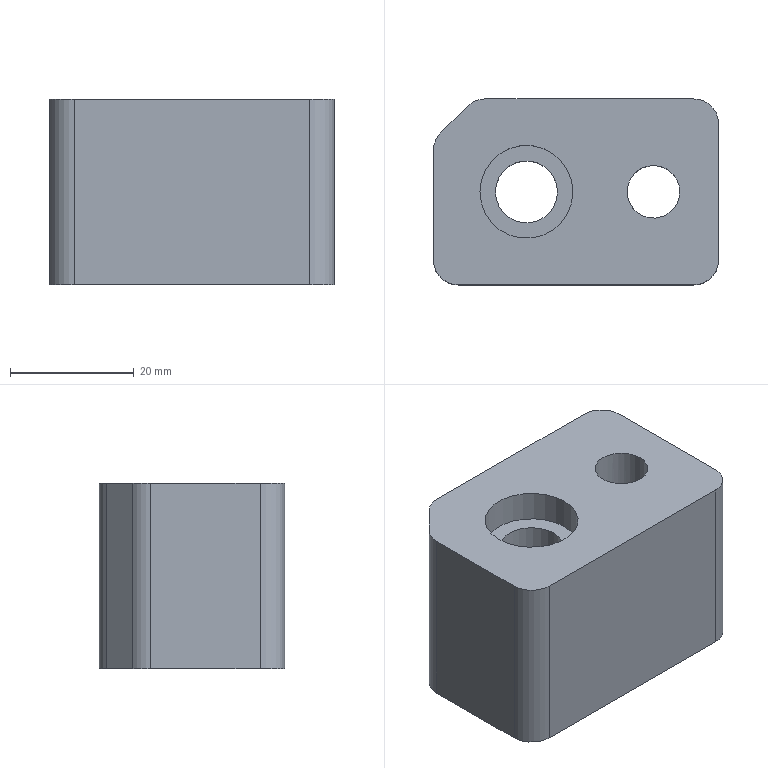Part | NX | features 7 2 | 1 solid | 18 faces | box 46 x 30 x 30 mm | volume 34235 mm3 | plane 9 | cylinder 9 | commonest cylinder face diameters 8 x5 8.5 x1 10 x1 14.5 x1 15 x1
STEP:
#1=CARTESIAN_POINT('',(3297.747,77.328,91.));
#2=VERTEX_POINT('',#1);
#3=CARTESIAN_POINT('',(3290.247,77.328,91.));
#4=DIRECTION('',(0.,0.,1.));
#5=DIRECTION('',(1.,0.,0.));
#6=AXIS2_PLACEMENT_3D('',#3,#4,#5);
#7=CIRCLE('',#6,7.5);
#8=EDGE_CURVE('',#2,#2,#7,.T.);
#9=ORIENTED_EDGE('',*,*,#8,.F.);
#10=EDGE_LOOP('',(#9));
#11=FACE_BOUND('',#10,.T.);
#12=CARTESIAN_POINT('',(3317.247,62.328,91.));
#13=VERTEX_POINT('',#12);
#14=CARTESIAN_POINT('',(3279.247,62.328,91.));
#15=VERTEX_POINT('',#14);
#16=CARTESIAN_POINT('',(3290.247,62.328,91.));
#17=DIRECTION('',(-1.,0.,0.));
#18=VECTOR('',#17,1000.);
#19=LINE('',#16,#18);
#20=EDGE_CURVE('',#13,#15,#19,.T.);
#21=ORIENTED_EDGE('',*,*,#20,.F.);
#22=CARTESIAN_POINT('',(3321.247,66.328,91.));
#23=VERTEX_POINT('',#22);
#24=CARTESIAN_POINT('',(3317.247,66.328,91.));
#25=DIRECTION('',(0.,0.,1.));
#26=DIRECTION('',(0.,1.,0.));
#27=AXIS2_PLACEMENT_3D('',#24,#25,#26);
#28=CIRCLE('',#27,4.);
#29=EDGE_CURVE('',#13,#23,#28,.T.);
#30=ORIENTED_EDGE('',*,*,#29,.T.);
#31=CARTESIAN_POINT('',(3321.247,88.328,91.));
#32=VERTEX_POINT('',#31);
#33=CARTESIAN_POINT('',(3321.247,77.328,91.));
#34=DIRECTION('',(0.,-1.,0.));
#35=VECTOR('',#34,1000.);
#36=LINE('',#33,#35);
#37=EDGE_CURVE('',#32,#23,#36,.T.);
#38=ORIENTED_EDGE('',*,*,#37,.F.);
#39=CARTESIAN_POINT('',(3317.247,92.328,91.));
#40=VERTEX_POINT('',#39);
#41=CARTESIAN_POINT('',(3317.247,88.328,91.));
#42=DIRECTION('',(0.,0.,1.));
#43=DIRECTION('',(0.,1.,0.));
#44=AXIS2_PLACEMENT_3D('',#41,#42,#43);
#45=CIRCLE('',#44,4.);
#46=EDGE_CURVE('',#32,#40,#45,.T.);
#47=ORIENTED_EDGE('',*,*,#46,.T.);
#48=CARTESIAN_POINT('',(3283.54,92.328,91.));
#49=VERTEX_POINT('',#48);
#50=CARTESIAN_POINT('',(3290.247,92.328,91.));
#51=DIRECTION('',(1.,0.,0.));
#52=VECTOR('',#51,1000.);
#53=LINE('',#50,#52);
#54=EDGE_CURVE('',#49,#40,#53,.T.);
#55=ORIENTED_EDGE('',*,*,#54,.F.);
#56=CARTESIAN_POINT('',(3280.711,91.157,91.));
#57=VERTEX_POINT('',#56);
#58=CARTESIAN_POINT('',(3283.54,88.328,91.));
#59=DIRECTION('',(0.,0.,1.));
#60=DIRECTION('',(0.,1.,0.));
#61=AXIS2_PLACEMENT_3D('',#58,#59,#60);
#62=CIRCLE('',#61,4.);
#63=EDGE_CURVE('',#49,#57,#62,.T.);
#64=ORIENTED_EDGE('',*,*,#63,.T.);
#65=CARTESIAN_POINT('',(3276.419,86.864,91.));
#66=VERTEX_POINT('',#65);
#67=CARTESIAN_POINT('',(3279.815,90.26,91.));
#68=DIRECTION('',(-0.7071,-0.7071,0.));
#69=VECTOR('',#68,1000.);
#70=LINE('',#67,#69);
#71=EDGE_CURVE('',#57,#66,#70,.T.);
#72=ORIENTED_EDGE('',*,*,#71,.T.);
#73=CARTESIAN_POINT('',(3275.247,84.035,91.));
#74=VERTEX_POINT('',#73);
#75=CARTESIAN_POINT('',(3279.247,84.035,91.));
#76=DIRECTION('',(0.,0.,1.));
#77=DIRECTION('',(0.,1.,0.));
#78=AXIS2_PLACEMENT_3D('',#75,#76,#77);
#79=CIRCLE('',#78,4.);
#80=EDGE_CURVE('',#66,#74,#79,.T.);
#81=ORIENTED_EDGE('',*,*,#80,.T.);
#82=CARTESIAN_POINT('',(3275.247,66.328,91.));
#83=VERTEX_POINT('',#82);
#84=CARTESIAN_POINT('',(3275.247,77.328,91.));
#85=DIRECTION('',(0.,1.,0.));
#86=VECTOR('',#85,1000.);
#87=LINE('',#84,#86);
#88=EDGE_CURVE('',#83,#74,#87,.T.);
#89=ORIENTED_EDGE('',*,*,#88,.F.);
#90=CARTESIAN_POINT('',(3279.247,66.328,91.));
#91=DIRECTION('',(0.,0.,1.));
#92=DIRECTION('',(0.,1.,0.));
#93=AXIS2_PLACEMENT_3D('',#90,#91,#92);
#94=CIRCLE('',#93,4.);
#95=EDGE_CURVE('',#83,#15,#94,.T.);
#96=ORIENTED_EDGE('',*,*,#95,.T.);
#97=EDGE_LOOP('',(#21,#30,#38,#47,#55,#64,#72,#81,#89,#96));
#98=FACE_BOUND('',#97,.T.);
#99=CARTESIAN_POINT('',(3310.747,81.578,91.));
#100=VERTEX_POINT('',#99);
#101=CARTESIAN_POINT('',(3310.747,77.328,91.));
#102=DIRECTION('',(0.,0.,-1.));
#103=DIRECTION('',(0.,1.,0.));
#104=AXIS2_PLACEMENT_3D('',#101,#102,#103);
#105=CIRCLE('',#104,4.25);
#106=EDGE_CURVE('',#100,#100,#105,.T.);
#107=ORIENTED_EDGE('',*,*,#106,.T.);
#108=EDGE_LOOP('',(#107));
#109=FACE_BOUND('',#108,.T.);
#110=CARTESIAN_POINT('',(3292.747,77.328,91.));
#111=DIRECTION('',(0.,0.,1.));
#112=DIRECTION('',(0.,-1.,0.));
#113=AXIS2_PLACEMENT_3D('',#110,#111,#112);
#114=PLANE('',#113);
#115=ADVANCED_FACE('',(#11,#98,#109),#114,.T.);
#116=CARTESIAN_POINT('',(3285.247,77.328,61.));
#117=VERTEX_POINT('',#116);
#118=CARTESIAN_POINT('',(3290.247,77.328,61.));
#119=DIRECTION('',(0.,0.,-1.));
#120=DIRECTION('',(-1.,0.,0.));
#121=AXIS2_PLACEMENT_3D('',#118,#119,#120);
#122=CIRCLE('',#121,5.);
#123=EDGE_CURVE('',#117,#117,#122,.T.);
#124=ORIENTED_EDGE('',*,*,#123,.F.);
#125=EDGE_LOOP('',(#124));
#126=FACE_BOUND('',#125,.T.);
#127=CARTESIAN_POINT('',(3303.497,77.328,61.));
#128=VERTEX_POINT('',#127);
#129=CARTESIAN_POINT('',(3310.747,77.328,61.));
#130=DIRECTION('',(0.,0.,-1.));
#131=DIRECTION('',(-1.,0.,0.));
#132=AXIS2_PLACEMENT_3D('',#129,#130,#131);
#133=CIRCLE('',#132,7.25);
#134=EDGE_CURVE('',#128,#128,#133,.T.);
#135=ORIENTED_EDGE('',*,*,#134,.F.);
#136=EDGE_LOOP('',(#135));
#137=FACE_BOUND('',#136,.T.);
#138=CARTESIAN_POINT('',(3321.247,66.328,61.));
#139=VERTEX_POINT('',#138);
#140=CARTESIAN_POINT('',(3321.247,88.328,61.));
#141=VERTEX_POINT('',#140);
#142=CARTESIAN_POINT('',(3321.247,-99.672,61.));
#143=DIRECTION('',(0.,1.,0.));
#144=VECTOR('',#143,1000.);
#145=LINE('',#142,#144);
#146=EDGE_CURVE('',#139,#141,#145,.T.);
#147=ORIENTED_EDGE('',*,*,#146,.F.);
#148=CARTESIAN_POINT('',(3317.247,62.328,61.));
#149=VERTEX_POINT('',#148);
#150=CARTESIAN_POINT('',(3317.247,66.328,61.));
#151=DIRECTION('',(0.,0.,-1.));
#152=DIRECTION('',(-1.,0.,0.));
#153=AXIS2_PLACEMENT_3D('',#150,#151,#152);
#154=CIRCLE('',#153,4.);
#155=EDGE_CURVE('',#139,#149,#154,.T.);
#156=ORIENTED_EDGE('',*,*,#155,.T.);
#157=CARTESIAN_POINT('',(3279.247,62.328,61.));
#158=VERTEX_POINT('',#157);
#159=CARTESIAN_POINT('',(3475.247,62.328,61.));
#160=DIRECTION('',(1.,0.,0.));
#161=VECTOR('',#160,1000.);
#162=LINE('',#159,#161);
#163=EDGE_CURVE('',#158,#149,#162,.T.);
#164=ORIENTED_EDGE('',*,*,#163,.F.);
#165=CARTESIAN_POINT('',(3275.247,66.328,61.));
#166=VERTEX_POINT('',#165);
#167=CARTESIAN_POINT('',(3279.247,66.328,61.));
#168=DIRECTION('',(0.,0.,-1.));
#169=DIRECTION('',(-1.,0.,0.));
#170=AXIS2_PLACEMENT_3D('',#167,#168,#169);
#171=CIRCLE('',#170,4.);
#172=EDGE_CURVE('',#158,#166,#171,.T.);
#173=ORIENTED_EDGE('',*,*,#172,.T.);
#174=CARTESIAN_POINT('',(3275.247,84.035,61.));
#175=VERTEX_POINT('',#174);
#176=CARTESIAN_POINT('',(3275.247,-99.672,61.));
#177=DIRECTION('',(0.,-1.,0.));
#178=VECTOR('',#177,1000.);
#179=LINE('',#176,#178);
#180=EDGE_CURVE('',#175,#166,#179,.T.);
#181=ORIENTED_EDGE('',*,*,#180,.F.);
#182=CARTESIAN_POINT('',(3276.419,86.864,61.));
#183=VERTEX_POINT('',#182);
#184=CARTESIAN_POINT('',(3279.247,84.035,61.));
#185=DIRECTION('',(0.,0.,-1.));
#186=DIRECTION('',(-1.,0.,0.));
#187=AXIS2_PLACEMENT_3D('',#184,#185,#186);
#188=CIRCLE('',#187,4.);
#189=EDGE_CURVE('',#175,#183,#188,.T.);
#190=ORIENTED_EDGE('',*,*,#189,.T.);
#191=CARTESIAN_POINT('',(3280.711,91.157,61.));
#192=VERTEX_POINT('',#191);
#193=CARTESIAN_POINT('',(3282.565,93.01,61.));
#194=DIRECTION('',(0.7071,0.7071,0.));
#195=VECTOR('',#194,1000.);
#196=LINE('',#193,#195);
#197=EDGE_CURVE('',#183,#192,#196,.T.);
#198=ORIENTED_EDGE('',*,*,#197,.T.);
#199=CARTESIAN_POINT('',(3283.54,92.328,61.));
#200=VERTEX_POINT('',#199);
#201=CARTESIAN_POINT('',(3283.54,88.328,61.));
#202=DIRECTION('',(0.,0.,-1.));
#203=DIRECTION('',(-1.,0.,0.));
#204=AXIS2_PLACEMENT_3D('',#201,#202,#203);
#205=CIRCLE('',#204,4.);
#206=EDGE_CURVE('',#192,#200,#205,.T.);
#207=ORIENTED_EDGE('',*,*,#206,.T.);
#208=CARTESIAN_POINT('',(3317.247,92.328,61.));
#209=VERTEX_POINT('',#208);
#210=CARTESIAN_POINT('',(3475.247,92.328,61.));
#211=DIRECTION('',(-1.,0.,0.));
#212=VECTOR('',#211,1000.);
#213=LINE('',#210,#212);
#214=EDGE_CURVE('',#209,#200,#213,.T.);
#215=ORIENTED_EDGE('',*,*,#214,.F.);
#216=CARTESIAN_POINT('',(3317.247,88.328,61.));
#217=DIRECTION('',(0.,0.,-1.));
#218=DIRECTION('',(-1.,0.,0.));
#219=AXIS2_PLACEMENT_3D('',#216,#217,#218);
#220=CIRCLE('',#219,4.);
#221=EDGE_CURVE('',#209,#141,#220,.T.);
#222=ORIENTED_EDGE('',*,*,#221,.T.);
#223=EDGE_LOOP('',(#147,#156,#164,#173,#181,#190,#198,#207,#215,#222));
#224=FACE_BOUND('',#223,.T.);
#225=CARTESIAN_POINT('',(3475.247,-99.672,61.));
#226=DIRECTION('',(0.,0.,-1.));
#227=DIRECTION('',(0.,1.,0.));
#228=AXIS2_PLACEMENT_3D('',#225,#226,#227);
#229=PLANE('',#228);
#230=ADVANCED_FACE('',(#126,#137,#224),#229,.T.);
#231=ORIENTED_EDGE('',*,*,#88,.T.);
#232=CARTESIAN_POINT('',(3275.247,84.035,-5.));
#233=DIRECTION('',(0.,0.,-1.));
#234=VECTOR('',#233,1000.);
#235=LINE('',#232,#234);
#236=EDGE_CURVE('',#74,#175,#235,.T.);
#237=ORIENTED_EDGE('',*,*,#236,.T.);
#238=ORIENTED_EDGE('',*,*,#180,.T.);
#239=CARTESIAN_POINT('',(3275.247,66.328,-5.));
#240=DIRECTION('',(0.,0.,1.));
#241=VECTOR('',#240,1000.);
#242=LINE('',#239,#241);
#243=EDGE_CURVE('',#166,#83,#242,.T.);
#244=ORIENTED_EDGE('',*,*,#243,.T.);
#245=EDGE_LOOP('',(#231,#237,#238,#244));
#246=FACE_BOUND('',#245,.T.);
#247=CARTESIAN_POINT('',(3275.247,77.328,-5.));
#248=DIRECTION('',(-1.,0.,0.));
#249=DIRECTION('',(0.,0.,-1.));
#250=AXIS2_PLACEMENT_3D('',#247,#248,#249);
#251=PLANE('',#250);
#252=ADVANCED_FACE('',(#246),#251,.T.);
#253=ORIENTED_EDGE('',*,*,#54,.T.);
#254=CARTESIAN_POINT('',(3317.247,92.328,-5.));
#255=DIRECTION('',(0.,0.,-1.));
#256=VECTOR('',#255,1000.);
#257=LINE('',#254,#256);
#258=EDGE_CURVE('',#40,#209,#257,.T.);
#259=ORIENTED_EDGE('',*,*,#258,.T.);
#260=ORIENTED_EDGE('',*,*,#214,.T.);
#261=CARTESIAN_POINT('',(3283.54,92.328,-5.));
#262=DIRECTION('',(0.,0.,1.));
#263=VECTOR('',#262,1000.);
#264=LINE('',#261,#263);
#265=EDGE_CURVE('',#200,#49,#264,.T.);
#266=ORIENTED_EDGE('',*,*,#265,.T.);
#267=EDGE_LOOP('',(#253,#259,#260,#266));
#268=FACE_BOUND('',#267,.T.);
#269=CARTESIAN_POINT('',(3290.247,92.328,-5.));
#270=DIRECTION('',(0.,1.,0.));
#271=DIRECTION('',(0.,0.,1.));
#272=AXIS2_PLACEMENT_3D('',#269,#270,#271);
#273=PLANE('',#272);
#274=ADVANCED_FACE('',(#268),#273,.T.);
#275=ORIENTED_EDGE('',*,*,#37,.T.);
#276=CARTESIAN_POINT('',(3321.247,66.328,-5.));
#277=DIRECTION('',(0.,0.,-1.));
#278=VECTOR('',#277,1000.);
#279=LINE('',#276,#278);
#280=EDGE_CURVE('',#23,#139,#279,.T.);
#281=ORIENTED_EDGE('',*,*,#280,.T.);
#282=ORIENTED_EDGE('',*,*,#146,.T.);
#283=CARTESIAN_POINT('',(3321.247,88.328,-5.));
#284=DIRECTION('',(0.,0.,1.));
#285=VECTOR('',#284,1000.);
#286=LINE('',#283,#285);
#287=EDGE_CURVE('',#141,#32,#286,.T.);
#288=ORIENTED_EDGE('',*,*,#287,.T.);
#289=EDGE_LOOP('',(#275,#281,#282,#288));
#290=FACE_BOUND('',#289,.T.);
#291=CARTESIAN_POINT('',(3321.247,77.328,-5.));
#292=DIRECTION('',(1.,0.,0.));
#293=DIRECTION('',(0.,0.,1.));
#294=AXIS2_PLACEMENT_3D('',#291,#292,#293);
#295=PLANE('',#294);
#296=ADVANCED_FACE('',(#290),#295,.T.);
#297=ORIENTED_EDGE('',*,*,#163,.T.);
#298=CARTESIAN_POINT('',(3317.247,62.328,-5.));
#299=DIRECTION('',(0.,0.,1.));
#300=VECTOR('',#299,1000.);
#301=LINE('',#298,#300);
#302=EDGE_CURVE('',#149,#13,#301,.T.);
#303=ORIENTED_EDGE('',*,*,#302,.T.);
#304=ORIENTED_EDGE('',*,*,#20,.T.);
#305=CARTESIAN_POINT('',(3279.247,62.328,-5.));
#306=DIRECTION('',(0.,0.,-1.));
#307=VECTOR('',#306,1000.);
#308=LINE('',#305,#307);
#309=EDGE_CURVE('',#15,#158,#308,.T.);
#310=ORIENTED_EDGE('',*,*,#309,.T.);
#311=EDGE_LOOP('',(#297,#303,#304,#310));
#312=FACE_BOUND('',#311,.T.);
#313=CARTESIAN_POINT('',(3290.247,62.328,-5.));
#314=DIRECTION('',(0.,-1.,0.));
#315=DIRECTION('',(0.,0.,-1.));
#316=AXIS2_PLACEMENT_3D('',#313,#314,#315);
#317=PLANE('',#316);
#318=ADVANCED_FACE('',(#312),#317,.T.);
#319=ORIENTED_EDGE('',*,*,#71,.F.);
#320=CARTESIAN_POINT('',(3280.711,91.157,-5.));
#321=DIRECTION('',(0.,0.,-1.));
#322=VECTOR('',#321,1000.);
#323=LINE('',#320,#322);
#324=EDGE_CURVE('',#57,#192,#323,.T.);
#325=ORIENTED_EDGE('',*,*,#324,.T.);
#326=ORIENTED_EDGE('',*,*,#197,.F.);
#327=CARTESIAN_POINT('',(3276.419,86.864,-5.));
#328=DIRECTION('',(0.,0.,1.));
#329=VECTOR('',#328,1000.);
#330=LINE('',#327,#329);
#331=EDGE_CURVE('',#183,#66,#330,.T.);
#332=ORIENTED_EDGE('',*,*,#331,.T.);
#333=EDGE_LOOP('',(#319,#325,#326,#332));
#334=FACE_BOUND('',#333,.T.);
#335=CARTESIAN_POINT('',(3282.565,93.01,-5.));
#336=DIRECTION('',(0.7071,-0.7071,0.));
#337=DIRECTION('',(0.,0.,1.));
#338=AXIS2_PLACEMENT_3D('',#335,#336,#337);
#339=PLANE('',#338);
#340=ADVANCED_FACE('',(#334),#339,.F.);
#341=ORIENTED_EDGE('',*,*,#155,.F.);
#342=ORIENTED_EDGE('',*,*,#280,.F.);
#343=ORIENTED_EDGE('',*,*,#29,.F.);
#344=ORIENTED_EDGE('',*,*,#302,.F.);
#345=EDGE_LOOP('',(#341,#342,#343,#344));
#346=FACE_BOUND('',#345,.T.);
#347=CARTESIAN_POINT('',(3317.247,66.328,-5.));
#348=DIRECTION('',(0.,0.,-1.));
#349=DIRECTION('',(0.,-1.,0.));
#350=AXIS2_PLACEMENT_3D('',#347,#348,#349);
#351=CYLINDRICAL_SURFACE('',#350,4.);
#352=ADVANCED_FACE('',(#346),#351,.T.);
#353=ORIENTED_EDGE('',*,*,#221,.F.);
#354=ORIENTED_EDGE('',*,*,#258,.F.);
#355=ORIENTED_EDGE('',*,*,#46,.F.);
#356=ORIENTED_EDGE('',*,*,#287,.F.);
#357=EDGE_LOOP('',(#353,#354,#355,#356));
#358=FACE_BOUND('',#357,.T.);
#359=CARTESIAN_POINT('',(3317.247,88.328,-5.));
#360=DIRECTION('',(0.,0.,-1.));
#361=DIRECTION('',(0.,-1.,0.));
#362=AXIS2_PLACEMENT_3D('',#359,#360,#361);
#363=CYLINDRICAL_SURFACE('',#362,4.);
#364=ADVANCED_FACE('',(#358),#363,.T.);
#365=ORIENTED_EDGE('',*,*,#206,.F.);
#366=ORIENTED_EDGE('',*,*,#324,.F.);
#367=ORIENTED_EDGE('',*,*,#63,.F.);
#368=ORIENTED_EDGE('',*,*,#265,.F.);
#369=EDGE_LOOP('',(#365,#366,#367,#368));
#370=FACE_BOUND('',#369,.T.);
#371=CARTESIAN_POINT('',(3283.54,88.328,-5.));
#372=DIRECTION('',(0.,0.,1.));
#373=DIRECTION('',(0.,1.,0.));
#374=AXIS2_PLACEMENT_3D('',#371,#372,#373);
#375=CYLINDRICAL_SURFACE('',#374,4.);
#376=ADVANCED_FACE('',(#370),#375,.T.);
#377=ORIENTED_EDGE('',*,*,#80,.F.);
#378=ORIENTED_EDGE('',*,*,#331,.F.);
#379=ORIENTED_EDGE('',*,*,#189,.F.);
#380=ORIENTED_EDGE('',*,*,#236,.F.);
#381=EDGE_LOOP('',(#377,#378,#379,#380));
#382=FACE_BOUND('',#381,.T.);
#383=CARTESIAN_POINT('',(3279.247,84.035,-5.));
#384=DIRECTION('',(0.,0.,-1.));
#385=DIRECTION('',(0.,-1.,0.));
#386=AXIS2_PLACEMENT_3D('',#383,#384,#385);
#387=CYLINDRICAL_SURFACE('',#386,4.);
#388=ADVANCED_FACE('',(#382),#387,.T.);
#389=ORIENTED_EDGE('',*,*,#172,.F.);
#390=ORIENTED_EDGE('',*,*,#309,.F.);
#391=ORIENTED_EDGE('',*,*,#95,.F.);
#392=ORIENTED_EDGE('',*,*,#243,.F.);
#393=EDGE_LOOP('',(#389,#390,#391,#392));
#394=FACE_BOUND('',#393,.T.);
#395=CARTESIAN_POINT('',(3279.247,66.328,-5.));
#396=DIRECTION('',(0.,0.,-1.));
#397=DIRECTION('',(0.,-1.,0.));
#398=AXIS2_PLACEMENT_3D('',#395,#396,#397);
#399=CYLINDRICAL_SURFACE('',#398,4.);
#400=ADVANCED_FACE('',(#394),#399,.T.);
#401=CARTESIAN_POINT('',(3314.997,77.328,76.));
#402=VERTEX_POINT('',#401);
#403=CARTESIAN_POINT('',(3310.747,77.328,76.));
#404=DIRECTION('',(0.,0.,1.));
#405=DIRECTION('',(1.,0.,0.));
#406=AXIS2_PLACEMENT_3D('',#403,#404,#405);
#407=CIRCLE('',#406,4.25);
#408=EDGE_CURVE('',#402,#402,#407,.T.);
#409=ORIENTED_EDGE('',*,*,#408,.F.);
#410=EDGE_LOOP('',(#409));
#411=FACE_BOUND('',#410,.T.);
#412=ORIENTED_EDGE('',*,*,#106,.F.);
#413=EDGE_LOOP('',(#412));
#414=FACE_BOUND('',#413,.T.);
#415=CARTESIAN_POINT('',(3310.747,77.328,55.));
#416=DIRECTION('',(0.,0.,1.));
#417=DIRECTION('',(0.,-1.,0.));
#418=AXIS2_PLACEMENT_3D('',#415,#416,#417);
#419=CYLINDRICAL_SURFACE('',#418,4.25);
#420=ADVANCED_FACE('',(#411,#414),#419,.F.);
#421=ORIENTED_EDGE('',*,*,#408,.T.);
#422=EDGE_LOOP('',(#421));
#423=FACE_BOUND('',#422,.T.);
#424=CARTESIAN_POINT('',(3317.997,77.328,76.));
#425=VERTEX_POINT('',#424);
#426=CARTESIAN_POINT('',(3310.747,77.328,76.));
#427=DIRECTION('',(0.,0.,1.));
#428=DIRECTION('',(1.,0.,0.));
#429=AXIS2_PLACEMENT_3D('',#426,#427,#428);
#430=CIRCLE('',#429,7.25);
#431=EDGE_CURVE('',#425,#425,#430,.T.);
#432=ORIENTED_EDGE('',*,*,#431,.F.);
#433=EDGE_LOOP('',(#432));
#434=FACE_BOUND('',#433,.T.);
#435=CARTESIAN_POINT('',(3310.747,77.328,76.));
#436=DIRECTION('',(0.,0.,1.));
#437=DIRECTION('',(0.,-1.,0.));
#438=AXIS2_PLACEMENT_3D('',#435,#436,#437);
#439=PLANE('',#438);
#440=ADVANCED_FACE('',(#423,#434),#439,.F.);
#441=ORIENTED_EDGE('',*,*,#134,.T.);
#442=EDGE_LOOP('',(#441));
#443=FACE_BOUND('',#442,.T.);
#444=ORIENTED_EDGE('',*,*,#431,.T.);
#445=EDGE_LOOP('',(#444));
#446=FACE_BOUND('',#445,.T.);
#447=CARTESIAN_POINT('',(3310.747,77.328,55.));
#448=DIRECTION('',(0.,0.,1.));
#449=DIRECTION('',(0.,-1.,0.));
#450=AXIS2_PLACEMENT_3D('',#447,#448,#449);
#451=CYLINDRICAL_SURFACE('',#450,7.25);
#452=ADVANCED_FACE('',(#443,#446),#451,.F.);
#453=CARTESIAN_POINT('',(3285.247,77.328,86.));
#454=VERTEX_POINT('',#453);
#455=CARTESIAN_POINT('',(3290.247,77.328,86.));
#456=DIRECTION('',(0.,0.,1.));
#457=DIRECTION('',(-1.,0.,0.));
#458=AXIS2_PLACEMENT_3D('',#455,#456,#457);
#459=CIRCLE('',#458,5.);
#460=EDGE_CURVE('',#454,#454,#459,.T.);
#461=ORIENTED_EDGE('',*,*,#460,.T.);
#462=EDGE_LOOP('',(#461));
#463=FACE_BOUND('',#462,.T.);
#464=ORIENTED_EDGE('',*,*,#123,.T.);
#465=EDGE_LOOP('',(#464));
#466=FACE_BOUND('',#465,.T.);
#467=CARTESIAN_POINT('',(3290.247,77.328,46.5));
#468=DIRECTION('',(0.,0.,-1.));
#469=DIRECTION('',(1.,0.,0.));
#470=AXIS2_PLACEMENT_3D('',#467,#468,#469);
#471=CYLINDRICAL_SURFACE('',#470,5.);
#472=ADVANCED_FACE('',(#463,#466),#471,.F.);
#473=CARTESIAN_POINT('',(3282.747,77.328,86.));
#474=VERTEX_POINT('',#473);
#475=CARTESIAN_POINT('',(3290.247,77.328,86.));
#476=DIRECTION('',(0.,0.,-1.));
#477=DIRECTION('',(-1.,0.,0.));
#478=AXIS2_PLACEMENT_3D('',#475,#476,#477);
#479=CIRCLE('',#478,7.5);
#480=EDGE_CURVE('',#474,#474,#479,.T.);
#481=ORIENTED_EDGE('',*,*,#480,.F.);
#482=EDGE_LOOP('',(#481));
#483=FACE_BOUND('',#482,.T.);
#484=ORIENTED_EDGE('',*,*,#460,.F.);
#485=EDGE_LOOP('',(#484));
#486=FACE_BOUND('',#485,.T.);
#487=CARTESIAN_POINT('',(3290.247,77.328,86.));
#488=DIRECTION('',(0.,0.,-1.));
#489=DIRECTION('',(0.,-1.,0.));
#490=AXIS2_PLACEMENT_3D('',#487,#488,#489);
#491=PLANE('',#490);
#492=ADVANCED_FACE('',(#483,#486),#491,.F.);
#493=ORIENTED_EDGE('',*,*,#8,.T.);
#494=EDGE_LOOP('',(#493));
#495=FACE_BOUND('',#494,.T.);
#496=ORIENTED_EDGE('',*,*,#480,.T.);
#497=EDGE_LOOP('',(#496));
#498=FACE_BOUND('',#497,.T.);
#499=CARTESIAN_POINT('',(3290.247,77.328,90.559));
#500=DIRECTION('',(0.,0.,-1.));
#501=DIRECTION('',(0.,1.,0.));
#502=AXIS2_PLACEMENT_3D('',#499,#500,#501);
#503=CYLINDRICAL_SURFACE('',#502,7.5);
#504=ADVANCED_FACE('',(#495,#498),#503,.F.);
#505=CLOSED_SHELL('',(#115,#230,#252,#274,#296,#318,#340,#352,#364,#376,#388,#400,#420,#440,#452,#472,#492,#504));
#506=MANIFOLD_SOLID_BREP('',#505);
#507=(LENGTH_UNIT()NAMED_UNIT(*)SI_UNIT(.MILLI.,.METRE.));
#508=UNCERTAINTY_MEASURE_WITH_UNIT(LENGTH_MEASURE(0.00001),#507,'','');
#509=(NAMED_UNIT(*)PLANE_ANGLE_UNIT()SI_UNIT($,.RADIAN.));
#510=(NAMED_UNIT(*)SI_UNIT($,.STERADIAN.)SOLID_ANGLE_UNIT());
#511=(GEOMETRIC_REPRESENTATION_CONTEXT(3)GLOBAL_UNCERTAINTY_ASSIGNED_CONTEXT((#508))GLOBAL_UNIT_ASSIGNED_CONTEXT((#507,#509,#510))REPRESENTATION_CONTEXT('',''));
#512=ADVANCED_BREP_SHAPE_REPRESENTATION('',(#506),#511);